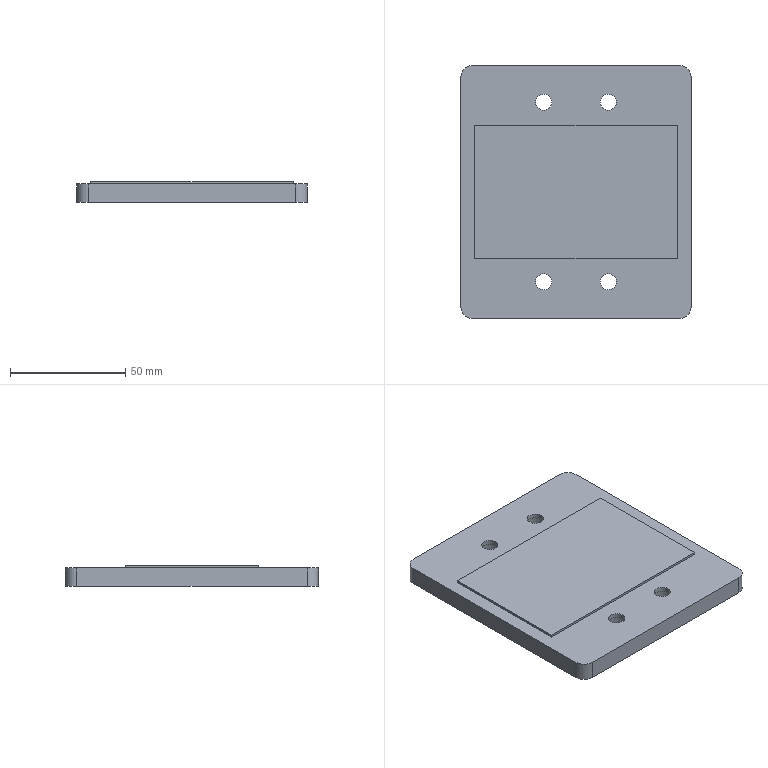Part | SolidWorks | features ICE 3, Extrusion 1 | 1 solid | 35 faces | box 100 x 110 x 9 mm | volume 89910 mm3 | cylinder 20 | plane 15 | commonest cylinder face diameters 7 x8 12 x8 10 x4
STEP:
#1=CARTESIAN_POINT('',(17.5,-39.,8.));
#2=VERTEX_POINT('',#1);
#3=CARTESIAN_POINT('',(10.5,-39.,8.));
#4=VERTEX_POINT('',#3);
#5=CARTESIAN_POINT('',(14.,-39.,8.));
#6=DIRECTION('',(0.,0.,-1.));
#7=DIRECTION('',(-1.,0.,0.));
#8=AXIS2_PLACEMENT_3D('',#5,#6,#7);
#9=CIRCLE('',#8,3.5);
#10=EDGE_CURVE('',#2,#4,#9,.T.);
#11=ORIENTED_EDGE('',*,*,#10,.F.);
#12=CARTESIAN_POINT('',(17.5,-39.,6.));
#13=VERTEX_POINT('',#12);
#14=CARTESIAN_POINT('',(17.5,-39.,12.));
#15=DIRECTION('',(0.,0.,-1.));
#16=VECTOR('',#15,1000.);
#17=LINE('',#14,#16);
#18=EDGE_CURVE('',#2,#13,#17,.T.);
#19=ORIENTED_EDGE('',*,*,#18,.T.);
#20=CARTESIAN_POINT('',(10.5,-39.,6.));
#21=VERTEX_POINT('',#20);
#22=CARTESIAN_POINT('',(14.,-39.,6.));
#23=DIRECTION('',(0.,0.,-1.));
#24=DIRECTION('',(1.,0.,0.));
#25=AXIS2_PLACEMENT_3D('',#22,#23,#24);
#26=CIRCLE('',#25,3.5);
#27=EDGE_CURVE('',#13,#21,#26,.T.);
#28=ORIENTED_EDGE('',*,*,#27,.T.);
#29=CARTESIAN_POINT('',(10.5,-39.,12.));
#30=DIRECTION('',(0.,0.,-1.));
#31=VECTOR('',#30,1000.);
#32=LINE('',#29,#31);
#33=EDGE_CURVE('',#4,#21,#32,.T.);
#34=ORIENTED_EDGE('',*,*,#33,.F.);
#35=EDGE_LOOP('',(#11,#19,#28,#34));
#36=FACE_OUTER_BOUND('',#35,.T.);
#37=CARTESIAN_POINT('',(14.,-39.,12.));
#38=DIRECTION('',(0.,0.,-1.));
#39=DIRECTION('',(-1.,0.,0.));
#40=AXIS2_PLACEMENT_3D('',#37,#38,#39);
#41=CYLINDRICAL_SURFACE('',#40,3.5);
#42=ADVANCED_FACE('',(#36),#41,.F.);
#43=CARTESIAN_POINT('',(-10.5,-39.,8.));
#44=VERTEX_POINT('',#43);
#45=CARTESIAN_POINT('',(-17.5,-39.,8.));
#46=VERTEX_POINT('',#45);
#47=CARTESIAN_POINT('',(-14.,-39.,8.));
#48=DIRECTION('',(0.,0.,-1.));
#49=DIRECTION('',(-1.,0.,0.));
#50=AXIS2_PLACEMENT_3D('',#47,#48,#49);
#51=CIRCLE('',#50,3.5);
#52=EDGE_CURVE('',#44,#46,#51,.T.);
#53=ORIENTED_EDGE('',*,*,#52,.F.);
#54=CARTESIAN_POINT('',(-10.5,-39.,6.));
#55=VERTEX_POINT('',#54);
#56=CARTESIAN_POINT('',(-10.5,-39.,12.));
#57=DIRECTION('',(0.,0.,-1.));
#58=VECTOR('',#57,1000.);
#59=LINE('',#56,#58);
#60=EDGE_CURVE('',#44,#55,#59,.T.);
#61=ORIENTED_EDGE('',*,*,#60,.T.);
#62=CARTESIAN_POINT('',(-17.5,-39.,6.));
#63=VERTEX_POINT('',#62);
#64=CARTESIAN_POINT('',(-14.,-39.,6.));
#65=DIRECTION('',(0.,0.,-1.));
#66=DIRECTION('',(1.,0.,0.));
#67=AXIS2_PLACEMENT_3D('',#64,#65,#66);
#68=CIRCLE('',#67,3.5);
#69=EDGE_CURVE('',#55,#63,#68,.T.);
#70=ORIENTED_EDGE('',*,*,#69,.T.);
#71=CARTESIAN_POINT('',(-17.5,-39.,12.));
#72=DIRECTION('',(0.,0.,-1.));
#73=VECTOR('',#72,1000.);
#74=LINE('',#71,#73);
#75=EDGE_CURVE('',#46,#63,#74,.T.);
#76=ORIENTED_EDGE('',*,*,#75,.F.);
#77=EDGE_LOOP('',(#53,#61,#70,#76));
#78=FACE_OUTER_BOUND('',#77,.T.);
#79=CARTESIAN_POINT('',(-14.,-39.,12.));
#80=DIRECTION('',(0.,0.,-1.));
#81=DIRECTION('',(-1.,0.,0.));
#82=AXIS2_PLACEMENT_3D('',#79,#80,#81);
#83=CYLINDRICAL_SURFACE('',#82,3.5);
#84=ADVANCED_FACE('',(#78),#83,.F.);
#85=CARTESIAN_POINT('',(-10.5,39.,8.));
#86=VERTEX_POINT('',#85);
#87=CARTESIAN_POINT('',(-17.5,39.,8.));
#88=VERTEX_POINT('',#87);
#89=CARTESIAN_POINT('',(-14.,39.,8.));
#90=DIRECTION('',(0.,0.,-1.));
#91=DIRECTION('',(-1.,0.,0.));
#92=AXIS2_PLACEMENT_3D('',#89,#90,#91);
#93=CIRCLE('',#92,3.5);
#94=EDGE_CURVE('',#86,#88,#93,.T.);
#95=ORIENTED_EDGE('',*,*,#94,.F.);
#96=CARTESIAN_POINT('',(-10.5,39.,6.));
#97=VERTEX_POINT('',#96);
#98=CARTESIAN_POINT('',(-10.5,39.,12.));
#99=DIRECTION('',(0.,0.,-1.));
#100=VECTOR('',#99,1000.);
#101=LINE('',#98,#100);
#102=EDGE_CURVE('',#86,#97,#101,.T.);
#103=ORIENTED_EDGE('',*,*,#102,.T.);
#104=CARTESIAN_POINT('',(-17.5,39.,6.));
#105=VERTEX_POINT('',#104);
#106=CARTESIAN_POINT('',(-14.,39.,6.));
#107=DIRECTION('',(0.,0.,-1.));
#108=DIRECTION('',(-1.,0.,0.));
#109=AXIS2_PLACEMENT_3D('',#106,#107,#108);
#110=CIRCLE('',#109,3.5);
#111=EDGE_CURVE('',#97,#105,#110,.T.);
#112=ORIENTED_EDGE('',*,*,#111,.T.);
#113=CARTESIAN_POINT('',(-17.5,39.,12.));
#114=DIRECTION('',(0.,0.,-1.));
#115=VECTOR('',#114,1000.);
#116=LINE('',#113,#115);
#117=EDGE_CURVE('',#88,#105,#116,.T.);
#118=ORIENTED_EDGE('',*,*,#117,.F.);
#119=EDGE_LOOP('',(#95,#103,#112,#118));
#120=FACE_OUTER_BOUND('',#119,.T.);
#121=CARTESIAN_POINT('',(-14.,39.,12.));
#122=DIRECTION('',(0.,0.,-1.));
#123=DIRECTION('',(-1.,0.,0.));
#124=AXIS2_PLACEMENT_3D('',#121,#122,#123);
#125=CYLINDRICAL_SURFACE('',#124,3.5);
#126=ADVANCED_FACE('',(#120),#125,.F.);
#127=CARTESIAN_POINT('',(17.5,39.,8.));
#128=VERTEX_POINT('',#127);
#129=CARTESIAN_POINT('',(10.5,39.,8.));
#130=VERTEX_POINT('',#129);
#131=CARTESIAN_POINT('',(14.,39.,8.));
#132=DIRECTION('',(0.,0.,-1.));
#133=DIRECTION('',(-1.,0.,0.));
#134=AXIS2_PLACEMENT_3D('',#131,#132,#133);
#135=CIRCLE('',#134,3.5);
#136=EDGE_CURVE('',#128,#130,#135,.T.);
#137=ORIENTED_EDGE('',*,*,#136,.F.);
#138=CARTESIAN_POINT('',(17.5,39.,6.));
#139=VERTEX_POINT('',#138);
#140=CARTESIAN_POINT('',(17.5,39.,12.));
#141=DIRECTION('',(0.,0.,-1.));
#142=VECTOR('',#141,1000.);
#143=LINE('',#140,#142);
#144=EDGE_CURVE('',#128,#139,#143,.T.);
#145=ORIENTED_EDGE('',*,*,#144,.T.);
#146=CARTESIAN_POINT('',(10.5,39.,6.));
#147=VERTEX_POINT('',#146);
#148=CARTESIAN_POINT('',(14.,39.,6.));
#149=DIRECTION('',(0.,0.,-1.));
#150=DIRECTION('',(-1.,0.,0.));
#151=AXIS2_PLACEMENT_3D('',#148,#149,#150);
#152=CIRCLE('',#151,3.5);
#153=EDGE_CURVE('',#139,#147,#152,.T.);
#154=ORIENTED_EDGE('',*,*,#153,.T.);
#155=CARTESIAN_POINT('',(10.5,39.,12.));
#156=DIRECTION('',(0.,0.,-1.));
#157=VECTOR('',#156,1000.);
#158=LINE('',#155,#157);
#159=EDGE_CURVE('',#130,#147,#158,.T.);
#160=ORIENTED_EDGE('',*,*,#159,.F.);
#161=EDGE_LOOP('',(#137,#145,#154,#160));
#162=FACE_OUTER_BOUND('',#161,.T.);
#163=CARTESIAN_POINT('',(14.,39.,12.));
#164=DIRECTION('',(0.,0.,-1.));
#165=DIRECTION('',(-1.,0.,0.));
#166=AXIS2_PLACEMENT_3D('',#163,#164,#165);
#167=CYLINDRICAL_SURFACE('',#166,3.5);
#168=ADVANCED_FACE('',(#162),#167,.F.);
#169=CARTESIAN_POINT('',(20.,39.,6.));
#170=VERTEX_POINT('',#169);
#171=CARTESIAN_POINT('',(8.,39.,6.));
#172=VERTEX_POINT('',#171);
#173=CARTESIAN_POINT('',(14.,39.,6.));
#174=DIRECTION('',(0.,0.,-1.));
#175=DIRECTION('',(1.,0.,0.));
#176=AXIS2_PLACEMENT_3D('',#173,#174,#175);
#177=CIRCLE('',#176,6.);
#178=EDGE_CURVE('',#170,#172,#177,.T.);
#179=ORIENTED_EDGE('',*,*,#178,.F.);
#180=CARTESIAN_POINT('',(20.,39.,0.));
#181=VERTEX_POINT('',#180);
#182=CARTESIAN_POINT('',(20.,39.,6.));
#183=DIRECTION('',(0.,0.,-1.));
#184=VECTOR('',#183,1000.);
#185=LINE('',#182,#184);
#186=EDGE_CURVE('',#170,#181,#185,.T.);
#187=ORIENTED_EDGE('',*,*,#186,.T.);
#188=CARTESIAN_POINT('',(8.,39.,0.));
#189=VERTEX_POINT('',#188);
#190=CARTESIAN_POINT('',(14.,39.,0.));
#191=DIRECTION('',(0.,0.,-1.));
#192=DIRECTION('',(1.,0.,0.));
#193=AXIS2_PLACEMENT_3D('',#190,#191,#192);
#194=CIRCLE('',#193,6.);
#195=EDGE_CURVE('',#181,#189,#194,.T.);
#196=ORIENTED_EDGE('',*,*,#195,.T.);
#197=CARTESIAN_POINT('',(8.,39.,6.));
#198=DIRECTION('',(0.,0.,-1.));
#199=VECTOR('',#198,1000.);
#200=LINE('',#197,#199);
#201=EDGE_CURVE('',#172,#189,#200,.T.);
#202=ORIENTED_EDGE('',*,*,#201,.F.);
#203=EDGE_LOOP('',(#179,#187,#196,#202));
#204=FACE_OUTER_BOUND('',#203,.T.);
#205=CARTESIAN_POINT('',(14.,39.,6.));
#206=DIRECTION('',(0.,0.,-1.));
#207=DIRECTION('',(-1.,0.,0.));
#208=AXIS2_PLACEMENT_3D('',#205,#206,#207);
#209=CYLINDRICAL_SURFACE('',#208,6.);
#210=ADVANCED_FACE('',(#204),#209,.F.);
#211=CARTESIAN_POINT('',(-8.,39.,6.));
#212=VERTEX_POINT('',#211);
#213=CARTESIAN_POINT('',(-20.,39.,6.));
#214=VERTEX_POINT('',#213);
#215=CARTESIAN_POINT('',(-14.,39.,6.));
#216=DIRECTION('',(0.,0.,-1.));
#217=DIRECTION('',(1.,0.,0.));
#218=AXIS2_PLACEMENT_3D('',#215,#216,#217);
#219=CIRCLE('',#218,6.);
#220=EDGE_CURVE('',#212,#214,#219,.T.);
#221=ORIENTED_EDGE('',*,*,#220,.F.);
#222=CARTESIAN_POINT('',(-8.,39.,0.));
#223=VERTEX_POINT('',#222);
#224=CARTESIAN_POINT('',(-8.,39.,6.));
#225=DIRECTION('',(0.,0.,-1.));
#226=VECTOR('',#225,1000.);
#227=LINE('',#224,#226);
#228=EDGE_CURVE('',#212,#223,#227,.T.);
#229=ORIENTED_EDGE('',*,*,#228,.T.);
#230=CARTESIAN_POINT('',(-20.,39.,0.));
#231=VERTEX_POINT('',#230);
#232=CARTESIAN_POINT('',(-14.,39.,0.));
#233=DIRECTION('',(0.,0.,-1.));
#234=DIRECTION('',(1.,0.,0.));
#235=AXIS2_PLACEMENT_3D('',#232,#233,#234);
#236=CIRCLE('',#235,6.);
#237=EDGE_CURVE('',#223,#231,#236,.T.);
#238=ORIENTED_EDGE('',*,*,#237,.T.);
#239=CARTESIAN_POINT('',(-20.,39.,6.));
#240=DIRECTION('',(0.,0.,-1.));
#241=VECTOR('',#240,1000.);
#242=LINE('',#239,#241);
#243=EDGE_CURVE('',#214,#231,#242,.T.);
#244=ORIENTED_EDGE('',*,*,#243,.F.);
#245=EDGE_LOOP('',(#221,#229,#238,#244));
#246=FACE_OUTER_BOUND('',#245,.T.);
#247=CARTESIAN_POINT('',(-14.,39.,6.));
#248=DIRECTION('',(0.,0.,-1.));
#249=DIRECTION('',(-1.,0.,0.));
#250=AXIS2_PLACEMENT_3D('',#247,#248,#249);
#251=CYLINDRICAL_SURFACE('',#250,6.);
#252=ADVANCED_FACE('',(#246),#251,.F.);
#253=CARTESIAN_POINT('',(-8.,-39.,6.));
#254=VERTEX_POINT('',#253);
#255=CARTESIAN_POINT('',(-20.,-39.,6.));
#256=VERTEX_POINT('',#255);
#257=CARTESIAN_POINT('',(-14.,-39.,6.));
#258=DIRECTION('',(0.,0.,-1.));
#259=DIRECTION('',(-1.,0.,0.));
#260=AXIS2_PLACEMENT_3D('',#257,#258,#259);
#261=CIRCLE('',#260,6.);
#262=EDGE_CURVE('',#254,#256,#261,.T.);
#263=ORIENTED_EDGE('',*,*,#262,.F.);
#264=CARTESIAN_POINT('',(-8.,-39.,0.));
#265=VERTEX_POINT('',#264);
#266=CARTESIAN_POINT('',(-8.,-39.,6.));
#267=DIRECTION('',(0.,0.,-1.));
#268=VECTOR('',#267,1000.);
#269=LINE('',#266,#268);
#270=EDGE_CURVE('',#254,#265,#269,.T.);
#271=ORIENTED_EDGE('',*,*,#270,.T.);
#272=CARTESIAN_POINT('',(-20.,-39.,0.));
#273=VERTEX_POINT('',#272);
#274=CARTESIAN_POINT('',(-14.,-39.,0.));
#275=DIRECTION('',(0.,0.,-1.));
#276=DIRECTION('',(-1.,0.,0.));
#277=AXIS2_PLACEMENT_3D('',#274,#275,#276);
#278=CIRCLE('',#277,6.);
#279=EDGE_CURVE('',#265,#273,#278,.T.);
#280=ORIENTED_EDGE('',*,*,#279,.T.);
#281=CARTESIAN_POINT('',(-20.,-39.,6.));
#282=DIRECTION('',(0.,0.,-1.));
#283=VECTOR('',#282,1000.);
#284=LINE('',#281,#283);
#285=EDGE_CURVE('',#256,#273,#284,.T.);
#286=ORIENTED_EDGE('',*,*,#285,.F.);
#287=EDGE_LOOP('',(#263,#271,#280,#286));
#288=FACE_OUTER_BOUND('',#287,.T.);
#289=CARTESIAN_POINT('',(-14.,-39.,6.));
#290=DIRECTION('',(0.,0.,-1.));
#291=DIRECTION('',(-1.,0.,0.));
#292=AXIS2_PLACEMENT_3D('',#289,#290,#291);
#293=CYLINDRICAL_SURFACE('',#292,6.);
#294=ADVANCED_FACE('',(#288),#293,.F.);
#295=CARTESIAN_POINT('',(20.,-39.,6.));
#296=VERTEX_POINT('',#295);
#297=CARTESIAN_POINT('',(8.,-39.,6.));
#298=VERTEX_POINT('',#297);
#299=CARTESIAN_POINT('',(14.,-39.,6.));
#300=DIRECTION('',(0.,0.,-1.));
#301=DIRECTION('',(-1.,0.,0.));
#302=AXIS2_PLACEMENT_3D('',#299,#300,#301);
#303=CIRCLE('',#302,6.);
#304=EDGE_CURVE('',#296,#298,#303,.T.);
#305=ORIENTED_EDGE('',*,*,#304,.F.);
#306=CARTESIAN_POINT('',(20.,-39.,0.));
#307=VERTEX_POINT('',#306);
#308=CARTESIAN_POINT('',(20.,-39.,6.));
#309=DIRECTION('',(0.,0.,-1.));
#310=VECTOR('',#309,1000.);
#311=LINE('',#308,#310);
#312=EDGE_CURVE('',#296,#307,#311,.T.);
#313=ORIENTED_EDGE('',*,*,#312,.T.);
#314=CARTESIAN_POINT('',(8.,-39.,0.));
#315=VERTEX_POINT('',#314);
#316=CARTESIAN_POINT('',(14.,-39.,0.));
#317=DIRECTION('',(0.,0.,-1.));
#318=DIRECTION('',(-1.,0.,0.));
#319=AXIS2_PLACEMENT_3D('',#316,#317,#318);
#320=CIRCLE('',#319,6.);
#321=EDGE_CURVE('',#307,#315,#320,.T.);
#322=ORIENTED_EDGE('',*,*,#321,.T.);
#323=CARTESIAN_POINT('',(8.,-39.,6.));
#324=DIRECTION('',(0.,0.,-1.));
#325=VECTOR('',#324,1000.);
#326=LINE('',#323,#325);
#327=EDGE_CURVE('',#298,#315,#326,.T.);
#328=ORIENTED_EDGE('',*,*,#327,.F.);
#329=EDGE_LOOP('',(#305,#313,#322,#328));
#330=FACE_OUTER_BOUND('',#329,.T.);
#331=CARTESIAN_POINT('',(14.,-39.,6.));
#332=DIRECTION('',(0.,0.,-1.));
#333=DIRECTION('',(-1.,0.,0.));
#334=AXIS2_PLACEMENT_3D('',#331,#332,#333);
#335=CYLINDRICAL_SURFACE('',#334,6.);
#336=ADVANCED_FACE('',(#330),#335,.F.);
#337=CARTESIAN_POINT('',(14.,-39.,8.));
#338=DIRECTION('',(0.,0.,-1.));
#339=DIRECTION('',(-1.,0.,0.));
#340=AXIS2_PLACEMENT_3D('',#337,#338,#339);
#341=CIRCLE('',#340,3.5);
#342=EDGE_CURVE('',#4,#2,#341,.T.);
#343=ORIENTED_EDGE('',*,*,#342,.T.);
#344=ORIENTED_EDGE('',*,*,#10,.T.);
#345=EDGE_LOOP('',(#343,#344));
#346=FACE_BOUND('',#345,.T.);
#347=CARTESIAN_POINT('',(-14.,-39.,8.));
#348=DIRECTION('',(0.,0.,-1.));
#349=DIRECTION('',(-1.,0.,0.));
#350=AXIS2_PLACEMENT_3D('',#347,#348,#349);
#351=CIRCLE('',#350,3.5);
#352=EDGE_CURVE('',#46,#44,#351,.T.);
#353=ORIENTED_EDGE('',*,*,#352,.T.);
#354=ORIENTED_EDGE('',*,*,#52,.T.);
#355=EDGE_LOOP('',(#353,#354));
#356=FACE_BOUND('',#355,.T.);
#357=CARTESIAN_POINT('',(-14.,39.,8.));
#358=DIRECTION('',(0.,0.,-1.));
#359=DIRECTION('',(-1.,0.,0.));
#360=AXIS2_PLACEMENT_3D('',#357,#358,#359);
#361=CIRCLE('',#360,3.5);
#362=EDGE_CURVE('',#88,#86,#361,.T.);
#363=ORIENTED_EDGE('',*,*,#362,.T.);
#364=ORIENTED_EDGE('',*,*,#94,.T.);
#365=EDGE_LOOP('',(#363,#364));
#366=FACE_BOUND('',#365,.T.);
#367=CARTESIAN_POINT('',(14.,39.,8.));
#368=DIRECTION('',(0.,0.,-1.));
#369=DIRECTION('',(-1.,0.,0.));
#370=AXIS2_PLACEMENT_3D('',#367,#368,#369);
#371=CIRCLE('',#370,3.5);
#372=EDGE_CURVE('',#130,#128,#371,.T.);
#373=ORIENTED_EDGE('',*,*,#372,.T.);
#374=ORIENTED_EDGE('',*,*,#136,.T.);
#375=EDGE_LOOP('',(#373,#374));
#376=FACE_BOUND('',#375,.T.);
#377=CARTESIAN_POINT('',(-50.,-50.,8.));
#378=VERTEX_POINT('',#377);
#379=CARTESIAN_POINT('',(-45.,-55.,8.));
#380=VERTEX_POINT('',#379);
#381=CARTESIAN_POINT('',(-45.,-50.,8.));
#382=DIRECTION('',(0.,0.,1.));
#383=DIRECTION('',(-1.,0.,0.));
#384=AXIS2_PLACEMENT_3D('',#381,#382,#383);
#385=CIRCLE('',#384,5.);
#386=EDGE_CURVE('',#378,#380,#385,.T.);
#387=ORIENTED_EDGE('',*,*,#386,.T.);
#388=CARTESIAN_POINT('',(45.,-55.,8.));
#389=VERTEX_POINT('',#388);
#390=CARTESIAN_POINT('',(-45.,-55.,8.));
#391=DIRECTION('',(1.,0.,0.));
#392=VECTOR('',#391,1000.);
#393=LINE('',#390,#392);
#394=EDGE_CURVE('',#380,#389,#393,.T.);
#395=ORIENTED_EDGE('',*,*,#394,.T.);
#396=CARTESIAN_POINT('',(50.,-50.,8.));
#397=VERTEX_POINT('',#396);
#398=CARTESIAN_POINT('',(45.,-50.,8.));
#399=DIRECTION('',(0.,0.,1.));
#400=DIRECTION('',(1.,0.,0.));
#401=AXIS2_PLACEMENT_3D('',#398,#399,#400);
#402=CIRCLE('',#401,5.);
#403=EDGE_CURVE('',#389,#397,#402,.T.);
#404=ORIENTED_EDGE('',*,*,#403,.T.);
#405=CARTESIAN_POINT('',(50.,50.,8.));
#406=VERTEX_POINT('',#405);
#407=CARTESIAN_POINT('',(50.,-50.,8.));
#408=DIRECTION('',(0.,1.,0.));
#409=VECTOR('',#408,1000.);
#410=LINE('',#407,#409);
#411=EDGE_CURVE('',#397,#406,#410,.T.);
#412=ORIENTED_EDGE('',*,*,#411,.T.);
#413=CARTESIAN_POINT('',(45.,55.,8.));
#414=VERTEX_POINT('',#413);
#415=CARTESIAN_POINT('',(45.,50.,8.));
#416=DIRECTION('',(0.,0.,1.));
#417=DIRECTION('',(-1.,0.,0.));
#418=AXIS2_PLACEMENT_3D('',#415,#416,#417);
#419=CIRCLE('',#418,5.);
#420=EDGE_CURVE('',#406,#414,#419,.T.);
#421=ORIENTED_EDGE('',*,*,#420,.T.);
#422=CARTESIAN_POINT('',(-45.,55.,8.));
#423=VERTEX_POINT('',#422);
#424=CARTESIAN_POINT('',(-45.,55.,8.));
#425=DIRECTION('',(-1.,0.,0.));
#426=VECTOR('',#425,1000.);
#427=LINE('',#424,#426);
#428=EDGE_CURVE('',#414,#423,#427,.T.);
#429=ORIENTED_EDGE('',*,*,#428,.T.);
#430=CARTESIAN_POINT('',(-50.,50.,8.));
#431=VERTEX_POINT('',#430);
#432=CARTESIAN_POINT('',(-45.,50.,8.));
#433=DIRECTION('',(0.,0.,1.));
#434=DIRECTION('',(-1.,0.,0.));
#435=AXIS2_PLACEMENT_3D('',#432,#433,#434);
#436=CIRCLE('',#435,5.);
#437=EDGE_CURVE('',#423,#431,#436,.T.);
#438=ORIENTED_EDGE('',*,*,#437,.T.);
#439=CARTESIAN_POINT('',(-50.,-50.,8.));
#440=DIRECTION('',(0.,-1.,0.));
#441=VECTOR('',#440,1000.);
#442=LINE('',#439,#441);
#443=EDGE_CURVE('',#431,#378,#442,.T.);
#444=ORIENTED_EDGE('',*,*,#443,.T.);
#445=EDGE_LOOP('',(#387,#395,#404,#412,#421,#429,#438,#444));
#446=FACE_OUTER_BOUND('',#445,.T.);
#447=CARTESIAN_POINT('',(44.,-29.,8.));
#448=VERTEX_POINT('',#447);
#449=CARTESIAN_POINT('',(44.,29.,8.));
#450=VERTEX_POINT('',#449);
#451=CARTESIAN_POINT('',(44.,-29.,8.));
#452=DIRECTION('',(0.,1.,0.));
#453=VECTOR('',#452,1000.);
#454=LINE('',#451,#453);
#455=EDGE_CURVE('',#448,#450,#454,.T.);
#456=ORIENTED_EDGE('',*,*,#455,.F.);
#457=CARTESIAN_POINT('',(-44.,-29.,8.));
#458=VERTEX_POINT('',#457);
#459=CARTESIAN_POINT('',(-44.,-29.,8.));
#460=DIRECTION('',(1.,0.,0.));
#461=VECTOR('',#460,1000.);
#462=LINE('',#459,#461);
#463=EDGE_CURVE('',#458,#448,#462,.T.);
#464=ORIENTED_EDGE('',*,*,#463,.F.);
#465=CARTESIAN_POINT('',(-44.,29.,8.));
#466=VERTEX_POINT('',#465);
#467=CARTESIAN_POINT('',(-44.,-29.,8.));
#468=DIRECTION('',(0.,-1.,0.));
#469=VECTOR('',#468,1000.);
#470=LINE('',#467,#469);
#471=EDGE_CURVE('',#466,#458,#470,.T.);
#472=ORIENTED_EDGE('',*,*,#471,.F.);
#473=CARTESIAN_POINT('',(-44.,29.,8.));
#474=DIRECTION('',(-1.,0.,0.));
#475=VECTOR('',#474,1000.);
#476=LINE('',#473,#475);
#477=EDGE_CURVE('',#450,#466,#476,.T.);
#478=ORIENTED_EDGE('',*,*,#477,.F.);
#479=EDGE_LOOP('',(#456,#464,#472,#478));
#480=FACE_BOUND('',#479,.T.);
#481=CARTESIAN_POINT('',(-45.,-50.,8.));
#482=DIRECTION('',(0.,0.,-1.));
#483=DIRECTION('',(-1.,0.,0.));
#484=AXIS2_PLACEMENT_3D('',#481,#482,#483);
#485=PLANE('',#484);
#486=ADVANCED_FACE('',(#346,#356,#366,#376,#446,#480),#485,.F.);
#487=CARTESIAN_POINT('',(-50.,-50.,0.));
#488=VERTEX_POINT('',#487);
#489=CARTESIAN_POINT('',(-45.,-55.,0.));
#490=VERTEX_POINT('',#489);
#491=CARTESIAN_POINT('',(-45.,-50.,0.));
#492=DIRECTION('',(0.,0.,1.));
#493=DIRECTION('',(-1.,0.,0.));
#494=AXIS2_PLACEMENT_3D('',#491,#492,#493);
#495=CIRCLE('',#494,5.);
#496=EDGE_CURVE('',#488,#490,#495,.T.);
#497=ORIENTED_EDGE('',*,*,#496,.T.);
#498=CARTESIAN_POINT('',(-45.,-55.,8.));
#499=DIRECTION('',(0.,0.,-1.));
#500=VECTOR('',#499,1000.);
#501=LINE('',#498,#500);
#502=EDGE_CURVE('',#380,#490,#501,.T.);
#503=ORIENTED_EDGE('',*,*,#502,.F.);
#504=ORIENTED_EDGE('',*,*,#386,.F.);
#505=CARTESIAN_POINT('',(-50.,-50.,8.));
#506=DIRECTION('',(0.,0.,-1.));
#507=VECTOR('',#506,1000.);
#508=LINE('',#505,#507);
#509=EDGE_CURVE('',#378,#488,#508,.T.);
#510=ORIENTED_EDGE('',*,*,#509,.T.);
#511=EDGE_LOOP('',(#497,#503,#504,#510));
#512=FACE_OUTER_BOUND('',#511,.T.);
#513=CARTESIAN_POINT('',(-45.,-50.,8.));
#514=DIRECTION('',(0.,0.,-1.));
#515=DIRECTION('',(-1.,0.,0.));
#516=AXIS2_PLACEMENT_3D('',#513,#514,#515);
#517=CYLINDRICAL_SURFACE('',#516,5.);
#518=ADVANCED_FACE('',(#512),#517,.T.);
#519=CARTESIAN_POINT('',(45.,-55.,0.));
#520=VERTEX_POINT('',#519);
#521=CARTESIAN_POINT('',(-45.,-55.,0.));
#522=DIRECTION('',(1.,0.,0.));
#523=VECTOR('',#522,1000.);
#524=LINE('',#521,#523);
#525=EDGE_CURVE('',#490,#520,#524,.T.);
#526=ORIENTED_EDGE('',*,*,#525,.T.);
#527=CARTESIAN_POINT('',(45.,-55.,8.));
#528=DIRECTION('',(0.,0.,-1.));
#529=VECTOR('',#528,1000.);
#530=LINE('',#527,#529);
#531=EDGE_CURVE('',#389,#520,#530,.T.);
#532=ORIENTED_EDGE('',*,*,#531,.F.);
#533=ORIENTED_EDGE('',*,*,#394,.F.);
#534=ORIENTED_EDGE('',*,*,#502,.T.);
#535=EDGE_LOOP('',(#526,#532,#533,#534));
#536=FACE_OUTER_BOUND('',#535,.T.);
#537=CARTESIAN_POINT('',(-45.,-55.,8.));
#538=DIRECTION('',(0.,1.,0.));
#539=DIRECTION('',(0.,0.,1.));
#540=AXIS2_PLACEMENT_3D('',#537,#538,#539);
#541=PLANE('',#540);
#542=ADVANCED_FACE('',(#536),#541,.F.);
#543=CARTESIAN_POINT('',(50.,-50.,0.));
#544=VERTEX_POINT('',#543);
#545=CARTESIAN_POINT('',(45.,-50.,0.));
#546=DIRECTION('',(0.,0.,1.));
#547=DIRECTION('',(1.,0.,0.));
#548=AXIS2_PLACEMENT_3D('',#545,#546,#547);
#549=CIRCLE('',#548,5.);
#550=EDGE_CURVE('',#520,#544,#549,.T.);
#551=ORIENTED_EDGE('',*,*,#550,.T.);
#552=CARTESIAN_POINT('',(50.,-50.,8.));
#553=DIRECTION('',(0.,0.,-1.));
#554=VECTOR('',#553,1000.);
#555=LINE('',#552,#554);
#556=EDGE_CURVE('',#397,#544,#555,.T.);
#557=ORIENTED_EDGE('',*,*,#556,.F.);
#558=ORIENTED_EDGE('',*,*,#403,.F.);
#559=ORIENTED_EDGE('',*,*,#531,.T.);
#560=EDGE_LOOP('',(#551,#557,#558,#559));
#561=FACE_OUTER_BOUND('',#560,.T.);
#562=CARTESIAN_POINT('',(45.,-50.,8.));
#563=DIRECTION('',(0.,0.,-1.));
#564=DIRECTION('',(-1.,0.,0.));
#565=AXIS2_PLACEMENT_3D('',#562,#563,#564);
#566=CYLINDRICAL_SURFACE('',#565,5.);
#567=ADVANCED_FACE('',(#561),#566,.T.);
#568=CARTESIAN_POINT('',(50.,50.,0.));
#569=VERTEX_POINT('',#568);
#570=CARTESIAN_POINT('',(50.,-50.,0.));
#571=DIRECTION('',(0.,1.,0.));
#572=VECTOR('',#571,1000.);
#573=LINE('',#570,#572);
#574=EDGE_CURVE('',#544,#569,#573,.T.);
#575=ORIENTED_EDGE('',*,*,#574,.T.);
#576=CARTESIAN_POINT('',(50.,50.,8.));
#577=DIRECTION('',(0.,0.,-1.));
#578=VECTOR('',#577,1000.);
#579=LINE('',#576,#578);
#580=EDGE_CURVE('',#406,#569,#579,.T.);
#581=ORIENTED_EDGE('',*,*,#580,.F.);
#582=ORIENTED_EDGE('',*,*,#411,.F.);
#583=ORIENTED_EDGE('',*,*,#556,.T.);
#584=EDGE_LOOP('',(#575,#581,#582,#583));
#585=FACE_OUTER_BOUND('',#584,.T.);
#586=CARTESIAN_POINT('',(50.,-50.,8.));
#587=DIRECTION('',(-1.,0.,0.));
#588=DIRECTION('',(0.,0.,1.));
#589=AXIS2_PLACEMENT_3D('',#586,#587,#588);
#590=PLANE('',#589);
#591=ADVANCED_FACE('',(#585),#590,.F.);
#592=CARTESIAN_POINT('',(45.,55.,0.));
#593=VERTEX_POINT('',#592);
#594=CARTESIAN_POINT('',(45.,50.,0.));
#595=DIRECTION('',(0.,0.,1.));
#596=DIRECTION('',(-1.,0.,0.));
#597=AXIS2_PLACEMENT_3D('',#594,#595,#596);
#598=CIRCLE('',#597,5.);
#599=EDGE_CURVE('',#569,#593,#598,.T.);
#600=ORIENTED_EDGE('',*,*,#599,.T.);
#601=CARTESIAN_POINT('',(45.,55.,8.));
#602=DIRECTION('',(0.,0.,-1.));
#603=VECTOR('',#602,1000.);
#604=LINE('',#601,#603);
#605=EDGE_CURVE('',#414,#593,#604,.T.);
#606=ORIENTED_EDGE('',*,*,#605,.F.);
#607=ORIENTED_EDGE('',*,*,#420,.F.);
#608=ORIENTED_EDGE('',*,*,#580,.T.);
#609=EDGE_LOOP('',(#600,#606,#607,#608));
#610=FACE_OUTER_BOUND('',#609,.T.);
#611=CARTESIAN_POINT('',(45.,50.,8.));
#612=DIRECTION('',(0.,0.,-1.));
#613=DIRECTION('',(-1.,0.,0.));
#614=AXIS2_PLACEMENT_3D('',#611,#612,#613);
#615=CYLINDRICAL_SURFACE('',#614,5.);
#616=ADVANCED_FACE('',(#610),#615,.T.);
#617=CARTESIAN_POINT('',(-45.,55.,0.));
#618=VERTEX_POINT('',#617);
#619=CARTESIAN_POINT('',(-45.,55.,0.));
#620=DIRECTION('',(-1.,0.,0.));
#621=VECTOR('',#620,1000.);
#622=LINE('',#619,#621);
#623=EDGE_CURVE('',#593,#618,#622,.T.);
#624=ORIENTED_EDGE('',*,*,#623,.T.);
#625=CARTESIAN_POINT('',(-45.,55.,8.));
#626=DIRECTION('',(0.,0.,-1.));
#627=VECTOR('',#626,1000.);
#628=LINE('',#625,#627);
#629=EDGE_CURVE('',#423,#618,#628,.T.);
#630=ORIENTED_EDGE('',*,*,#629,.F.);
#631=ORIENTED_EDGE('',*,*,#428,.F.);
#632=ORIENTED_EDGE('',*,*,#605,.T.);
#633=EDGE_LOOP('',(#624,#630,#631,#632));
#634=FACE_OUTER_BOUND('',#633,.T.);
#635=CARTESIAN_POINT('',(-45.,55.,8.));
#636=DIRECTION('',(0.,-1.,0.));
#637=DIRECTION('',(0.,0.,-1.));
#638=AXIS2_PLACEMENT_3D('',#635,#636,#637);
#639=PLANE('',#638);
#640=ADVANCED_FACE('',(#634),#639,.F.);
#641=CARTESIAN_POINT('',(-50.,50.,0.));
#642=VERTEX_POINT('',#641);
#643=CARTESIAN_POINT('',(-45.,50.,0.));
#644=DIRECTION('',(0.,0.,1.));
#645=DIRECTION('',(-1.,0.,0.));
#646=AXIS2_PLACEMENT_3D('',#643,#644,#645);
#647=CIRCLE('',#646,5.);
#648=EDGE_CURVE('',#618,#642,#647,.T.);
#649=ORIENTED_EDGE('',*,*,#648,.T.);
#650=CARTESIAN_POINT('',(-50.,50.,8.));
#651=DIRECTION('',(0.,0.,-1.));
#652=VECTOR('',#651,1000.);
#653=LINE('',#650,#652);
#654=EDGE_CURVE('',#431,#642,#653,.T.);
#655=ORIENTED_EDGE('',*,*,#654,.F.);
#656=ORIENTED_EDGE('',*,*,#437,.F.);
#657=ORIENTED_EDGE('',*,*,#629,.T.);
#658=EDGE_LOOP('',(#649,#655,#656,#657));
#659=FACE_OUTER_BOUND('',#658,.T.);
#660=CARTESIAN_POINT('',(-45.,50.,8.));
#661=DIRECTION('',(0.,0.,-1.));
#662=DIRECTION('',(-1.,0.,0.));
#663=AXIS2_PLACEMENT_3D('',#660,#661,#662);
#664=CYLINDRICAL_SURFACE('',#663,5.);
#665=ADVANCED_FACE('',(#659),#664,.T.);
#666=CARTESIAN_POINT('',(-50.,-50.,0.));
#667=DIRECTION('',(0.,-1.,0.));
#668=VECTOR('',#667,1000.);
#669=LINE('',#666,#668);
#670=EDGE_CURVE('',#642,#488,#669,.T.);
#671=ORIENTED_EDGE('',*,*,#670,.T.);
#672=ORIENTED_EDGE('',*,*,#509,.F.);
#673=ORIENTED_EDGE('',*,*,#443,.F.);
#674=ORIENTED_EDGE('',*,*,#654,.T.);
#675=EDGE_LOOP('',(#671,#672,#673,#674));
#676=FACE_OUTER_BOUND('',#675,.T.);
#677=CARTESIAN_POINT('',(-50.,-50.,8.));
#678=DIRECTION('',(1.,0.,0.));
#679=DIRECTION('',(0.,0.,-1.));
#680=AXIS2_PLACEMENT_3D('',#677,#678,#679);
#681=PLANE('',#680);
#682=ADVANCED_FACE('',(#676),#681,.F.);
#683=CARTESIAN_POINT('',(14.,39.,0.));
#684=DIRECTION('',(0.,0.,-1.));
#685=DIRECTION('',(1.,0.,0.));
#686=AXIS2_PLACEMENT_3D('',#683,#684,#685);
#687=CIRCLE('',#686,6.);
#688=EDGE_CURVE('',#189,#181,#687,.T.);
#689=ORIENTED_EDGE('',*,*,#688,.F.);
#690=ORIENTED_EDGE('',*,*,#195,.F.);
#691=EDGE_LOOP('',(#689,#690));
#692=FACE_BOUND('',#691,.T.);
#693=CARTESIAN_POINT('',(-14.,39.,0.));
#694=DIRECTION('',(0.,0.,-1.));
#695=DIRECTION('',(1.,0.,0.));
#696=AXIS2_PLACEMENT_3D('',#693,#694,#695);
#697=CIRCLE('',#696,6.);
#698=EDGE_CURVE('',#231,#223,#697,.T.);
#699=ORIENTED_EDGE('',*,*,#698,.F.);
#700=ORIENTED_EDGE('',*,*,#237,.F.);
#701=EDGE_LOOP('',(#699,#700));
#702=FACE_BOUND('',#701,.T.);
#703=CARTESIAN_POINT('',(-14.,-39.,0.));
#704=DIRECTION('',(0.,0.,-1.));
#705=DIRECTION('',(-1.,0.,0.));
#706=AXIS2_PLACEMENT_3D('',#703,#704,#705);
#707=CIRCLE('',#706,6.);
#708=EDGE_CURVE('',#273,#265,#707,.T.);
#709=ORIENTED_EDGE('',*,*,#708,.F.);
#710=ORIENTED_EDGE('',*,*,#279,.F.);
#711=EDGE_LOOP('',(#709,#710));
#712=FACE_BOUND('',#711,.T.);
#713=CARTESIAN_POINT('',(14.,-39.,0.));
#714=DIRECTION('',(0.,0.,-1.));
#715=DIRECTION('',(-1.,0.,0.));
#716=AXIS2_PLACEMENT_3D('',#713,#714,#715);
#717=CIRCLE('',#716,6.);
#718=EDGE_CURVE('',#315,#307,#717,.T.);
#719=ORIENTED_EDGE('',*,*,#718,.F.);
#720=ORIENTED_EDGE('',*,*,#321,.F.);
#721=EDGE_LOOP('',(#719,#720));
#722=FACE_BOUND('',#721,.T.);
#723=ORIENTED_EDGE('',*,*,#496,.F.);
#724=ORIENTED_EDGE('',*,*,#670,.F.);
#725=ORIENTED_EDGE('',*,*,#648,.F.);
#726=ORIENTED_EDGE('',*,*,#623,.F.);
#727=ORIENTED_EDGE('',*,*,#599,.F.);
#728=ORIENTED_EDGE('',*,*,#574,.F.);
#729=ORIENTED_EDGE('',*,*,#550,.F.);
#730=ORIENTED_EDGE('',*,*,#525,.F.);
#731=EDGE_LOOP('',(#723,#724,#725,#726,#727,#728,#729,#730));
#732=FACE_OUTER_BOUND('',#731,.T.);
#733=CARTESIAN_POINT('',(-45.,-50.,0.));
#734=DIRECTION('',(0.,0.,-1.));
#735=DIRECTION('',(-1.,0.,0.));
#736=AXIS2_PLACEMENT_3D('',#733,#734,#735);
#737=PLANE('',#736);
#738=ADVANCED_FACE('',(#692,#702,#712,#722,#732),#737,.T.);
#739=ORIENTED_EDGE('',*,*,#455,.T.);
#740=CARTESIAN_POINT('',(44.,29.,9.));
#741=VERTEX_POINT('',#740);
#742=CARTESIAN_POINT('',(44.,29.,9.));
#743=DIRECTION('',(0.,0.,-1.));
#744=VECTOR('',#743,1000.);
#745=LINE('',#742,#744);
#746=EDGE_CURVE('',#741,#450,#745,.T.);
#747=ORIENTED_EDGE('',*,*,#746,.F.);
#748=CARTESIAN_POINT('',(44.,-29.,9.));
#749=VERTEX_POINT('',#748);
#750=CARTESIAN_POINT('',(44.,-29.,9.));
#751=DIRECTION('',(0.,1.,0.));
#752=VECTOR('',#751,1000.);
#753=LINE('',#750,#752);
#754=EDGE_CURVE('',#749,#741,#753,.T.);
#755=ORIENTED_EDGE('',*,*,#754,.F.);
#756=CARTESIAN_POINT('',(44.,-29.,9.));
#757=DIRECTION('',(0.,0.,-1.));
#758=VECTOR('',#757,1000.);
#759=LINE('',#756,#758);
#760=EDGE_CURVE('',#749,#448,#759,.T.);
#761=ORIENTED_EDGE('',*,*,#760,.T.);
#762=EDGE_LOOP('',(#739,#747,#755,#761));
#763=FACE_OUTER_BOUND('',#762,.T.);
#764=CARTESIAN_POINT('',(44.,-29.,9.));
#765=DIRECTION('',(-1.,0.,0.));
#766=DIRECTION('',(0.,0.,1.));
#767=AXIS2_PLACEMENT_3D('',#764,#765,#766);
#768=PLANE('',#767);
#769=ADVANCED_FACE('',(#763),#768,.F.);
#770=ORIENTED_EDGE('',*,*,#477,.T.);
#771=CARTESIAN_POINT('',(-44.,29.,9.));
#772=VERTEX_POINT('',#771);
#773=CARTESIAN_POINT('',(-44.,29.,9.));
#774=DIRECTION('',(0.,0.,-1.));
#775=VECTOR('',#774,1000.);
#776=LINE('',#773,#775);
#777=EDGE_CURVE('',#772,#466,#776,.T.);
#778=ORIENTED_EDGE('',*,*,#777,.F.);
#779=CARTESIAN_POINT('',(-44.,29.,9.));
#780=DIRECTION('',(-1.,0.,0.));
#781=VECTOR('',#780,1000.);
#782=LINE('',#779,#781);
#783=EDGE_CURVE('',#741,#772,#782,.T.);
#784=ORIENTED_EDGE('',*,*,#783,.F.);
#785=ORIENTED_EDGE('',*,*,#746,.T.);
#786=EDGE_LOOP('',(#770,#778,#784,#785));
#787=FACE_OUTER_BOUND('',#786,.T.);
#788=CARTESIAN_POINT('',(-44.,29.,9.));
#789=DIRECTION('',(0.,-1.,0.));
#790=DIRECTION('',(0.,0.,-1.));
#791=AXIS2_PLACEMENT_3D('',#788,#789,#790);
#792=PLANE('',#791);
#793=ADVANCED_FACE('',(#787),#792,.F.);
#794=ORIENTED_EDGE('',*,*,#471,.T.);
#795=CARTESIAN_POINT('',(-44.,-29.,9.));
#796=VERTEX_POINT('',#795);
#797=CARTESIAN_POINT('',(-44.,-29.,9.));
#798=DIRECTION('',(0.,0.,-1.));
#799=VECTOR('',#798,1000.);
#800=LINE('',#797,#799);
#801=EDGE_CURVE('',#796,#458,#800,.T.);
#802=ORIENTED_EDGE('',*,*,#801,.F.);
#803=CARTESIAN_POINT('',(-44.,-29.,9.));
#804=DIRECTION('',(0.,-1.,0.));
#805=VECTOR('',#804,1000.);
#806=LINE('',#803,#805);
#807=EDGE_CURVE('',#772,#796,#806,.T.);
#808=ORIENTED_EDGE('',*,*,#807,.F.);
#809=ORIENTED_EDGE('',*,*,#777,.T.);
#810=EDGE_LOOP('',(#794,#802,#808,#809));
#811=FACE_OUTER_BOUND('',#810,.T.);
#812=CARTESIAN_POINT('',(-44.,-29.,9.));
#813=DIRECTION('',(1.,0.,0.));
#814=DIRECTION('',(0.,0.,-1.));
#815=AXIS2_PLACEMENT_3D('',#812,#813,#814);
#816=PLANE('',#815);
#817=ADVANCED_FACE('',(#811),#816,.F.);
#818=ORIENTED_EDGE('',*,*,#463,.T.);
#819=ORIENTED_EDGE('',*,*,#760,.F.);
#820=CARTESIAN_POINT('',(-44.,-29.,9.));
#821=DIRECTION('',(1.,0.,0.));
#822=VECTOR('',#821,1000.);
#823=LINE('',#820,#822);
#824=EDGE_CURVE('',#796,#749,#823,.T.);
#825=ORIENTED_EDGE('',*,*,#824,.F.);
#826=ORIENTED_EDGE('',*,*,#801,.T.);
#827=EDGE_LOOP('',(#818,#819,#825,#826));
#828=FACE_OUTER_BOUND('',#827,.T.);
#829=CARTESIAN_POINT('',(-44.,-29.,9.));
#830=DIRECTION('',(0.,1.,0.));
#831=DIRECTION('',(0.,0.,1.));
#832=AXIS2_PLACEMENT_3D('',#829,#830,#831);
#833=PLANE('',#832);
#834=ADVANCED_FACE('',(#828),#833,.F.);
#835=ORIENTED_EDGE('',*,*,#754,.T.);
#836=ORIENTED_EDGE('',*,*,#783,.T.);
#837=ORIENTED_EDGE('',*,*,#807,.T.);
#838=ORIENTED_EDGE('',*,*,#824,.T.);
#839=EDGE_LOOP('',(#835,#836,#837,#838));
#840=FACE_OUTER_BOUND('',#839,.T.);
#841=CARTESIAN_POINT('',(0.,0.,9.));
#842=DIRECTION('',(0.,0.,-1.));
#843=DIRECTION('',(-1.,0.,0.));
#844=AXIS2_PLACEMENT_3D('',#841,#842,#843);
#845=PLANE('',#844);
#846=ADVANCED_FACE('',(#840),#845,.F.);
#847=ORIENTED_EDGE('',*,*,#312,.F.);
#848=CARTESIAN_POINT('',(14.,-39.,6.));
#849=DIRECTION('',(0.,0.,-1.));
#850=DIRECTION('',(-1.,0.,0.));
#851=AXIS2_PLACEMENT_3D('',#848,#849,#850);
#852=CIRCLE('',#851,6.);
#853=EDGE_CURVE('',#298,#296,#852,.T.);
#854=ORIENTED_EDGE('',*,*,#853,.F.);
#855=ORIENTED_EDGE('',*,*,#327,.T.);
#856=ORIENTED_EDGE('',*,*,#718,.T.);
#857=EDGE_LOOP('',(#847,#854,#855,#856));
#858=FACE_OUTER_BOUND('',#857,.T.);
#859=CARTESIAN_POINT('',(14.,-39.,6.));
#860=DIRECTION('',(0.,0.,-1.));
#861=DIRECTION('',(-1.,0.,0.));
#862=AXIS2_PLACEMENT_3D('',#859,#860,#861);
#863=CYLINDRICAL_SURFACE('',#862,6.);
#864=ADVANCED_FACE('',(#858),#863,.F.);
#865=CARTESIAN_POINT('',(14.,-39.,6.));
#866=DIRECTION('',(0.,0.,-1.));
#867=DIRECTION('',(1.,0.,0.));
#868=AXIS2_PLACEMENT_3D('',#865,#866,#867);
#869=CIRCLE('',#868,3.5);
#870=EDGE_CURVE('',#21,#13,#869,.T.);
#871=ORIENTED_EDGE('',*,*,#870,.F.);
#872=ORIENTED_EDGE('',*,*,#27,.F.);
#873=EDGE_LOOP('',(#871,#872));
#874=FACE_BOUND('',#873,.T.);
#875=ORIENTED_EDGE('',*,*,#853,.T.);
#876=ORIENTED_EDGE('',*,*,#304,.T.);
#877=EDGE_LOOP('',(#875,#876));
#878=FACE_OUTER_BOUND('',#877,.T.);
#879=CARTESIAN_POINT('',(14.,-39.,6.));
#880=DIRECTION('',(0.,0.,-1.));
#881=DIRECTION('',(-1.,0.,0.));
#882=AXIS2_PLACEMENT_3D('',#879,#880,#881);
#883=PLANE('',#882);
#884=ADVANCED_FACE('',(#874,#878),#883,.T.);
#885=ORIENTED_EDGE('',*,*,#270,.F.);
#886=CARTESIAN_POINT('',(-14.,-39.,6.));
#887=DIRECTION('',(0.,0.,-1.));
#888=DIRECTION('',(-1.,0.,0.));
#889=AXIS2_PLACEMENT_3D('',#886,#887,#888);
#890=CIRCLE('',#889,6.);
#891=EDGE_CURVE('',#256,#254,#890,.T.);
#892=ORIENTED_EDGE('',*,*,#891,.F.);
#893=ORIENTED_EDGE('',*,*,#285,.T.);
#894=ORIENTED_EDGE('',*,*,#708,.T.);
#895=EDGE_LOOP('',(#885,#892,#893,#894));
#896=FACE_OUTER_BOUND('',#895,.T.);
#897=CARTESIAN_POINT('',(-14.,-39.,6.));
#898=DIRECTION('',(0.,0.,-1.));
#899=DIRECTION('',(-1.,0.,0.));
#900=AXIS2_PLACEMENT_3D('',#897,#898,#899);
#901=CYLINDRICAL_SURFACE('',#900,6.);
#902=ADVANCED_FACE('',(#896),#901,.F.);
#903=CARTESIAN_POINT('',(-14.,-39.,6.));
#904=DIRECTION('',(0.,0.,-1.));
#905=DIRECTION('',(1.,0.,0.));
#906=AXIS2_PLACEMENT_3D('',#903,#904,#905);
#907=CIRCLE('',#906,3.5);
#908=EDGE_CURVE('',#63,#55,#907,.T.);
#909=ORIENTED_EDGE('',*,*,#908,.F.);
#910=ORIENTED_EDGE('',*,*,#69,.F.);
#911=EDGE_LOOP('',(#909,#910));
#912=FACE_BOUND('',#911,.T.);
#913=ORIENTED_EDGE('',*,*,#891,.T.);
#914=ORIENTED_EDGE('',*,*,#262,.T.);
#915=EDGE_LOOP('',(#913,#914));
#916=FACE_OUTER_BOUND('',#915,.T.);
#917=CARTESIAN_POINT('',(-14.,-39.,6.));
#918=DIRECTION('',(0.,0.,-1.));
#919=DIRECTION('',(-1.,0.,0.));
#920=AXIS2_PLACEMENT_3D('',#917,#918,#919);
#921=PLANE('',#920);
#922=ADVANCED_FACE('',(#912,#916),#921,.T.);
#923=ORIENTED_EDGE('',*,*,#228,.F.);
#924=CARTESIAN_POINT('',(-14.,39.,6.));
#925=DIRECTION('',(0.,0.,-1.));
#926=DIRECTION('',(1.,0.,0.));
#927=AXIS2_PLACEMENT_3D('',#924,#925,#926);
#928=CIRCLE('',#927,6.);
#929=EDGE_CURVE('',#214,#212,#928,.T.);
#930=ORIENTED_EDGE('',*,*,#929,.F.);
#931=ORIENTED_EDGE('',*,*,#243,.T.);
#932=ORIENTED_EDGE('',*,*,#698,.T.);
#933=EDGE_LOOP('',(#923,#930,#931,#932));
#934=FACE_OUTER_BOUND('',#933,.T.);
#935=CARTESIAN_POINT('',(-14.,39.,6.));
#936=DIRECTION('',(0.,0.,-1.));
#937=DIRECTION('',(-1.,0.,0.));
#938=AXIS2_PLACEMENT_3D('',#935,#936,#937);
#939=CYLINDRICAL_SURFACE('',#938,6.);
#940=ADVANCED_FACE('',(#934),#939,.F.);
#941=CARTESIAN_POINT('',(-14.,39.,6.));
#942=DIRECTION('',(0.,0.,-1.));
#943=DIRECTION('',(-1.,0.,0.));
#944=AXIS2_PLACEMENT_3D('',#941,#942,#943);
#945=CIRCLE('',#944,3.5);
#946=EDGE_CURVE('',#105,#97,#945,.T.);
#947=ORIENTED_EDGE('',*,*,#946,.F.);
#948=ORIENTED_EDGE('',*,*,#111,.F.);
#949=EDGE_LOOP('',(#947,#948));
#950=FACE_BOUND('',#949,.T.);
#951=ORIENTED_EDGE('',*,*,#929,.T.);
#952=ORIENTED_EDGE('',*,*,#220,.T.);
#953=EDGE_LOOP('',(#951,#952));
#954=FACE_OUTER_BOUND('',#953,.T.);
#955=CARTESIAN_POINT('',(-14.,39.,6.));
#956=DIRECTION('',(0.,0.,1.));
#957=DIRECTION('',(1.,0.,0.));
#958=AXIS2_PLACEMENT_3D('',#955,#956,#957);
#959=PLANE('',#958);
#960=ADVANCED_FACE('',(#950,#954),#959,.F.);
#961=ORIENTED_EDGE('',*,*,#186,.F.);
#962=CARTESIAN_POINT('',(14.,39.,6.));
#963=DIRECTION('',(0.,0.,-1.));
#964=DIRECTION('',(1.,0.,0.));
#965=AXIS2_PLACEMENT_3D('',#962,#963,#964);
#966=CIRCLE('',#965,6.);
#967=EDGE_CURVE('',#172,#170,#966,.T.);
#968=ORIENTED_EDGE('',*,*,#967,.F.);
#969=ORIENTED_EDGE('',*,*,#201,.T.);
#970=ORIENTED_EDGE('',*,*,#688,.T.);
#971=EDGE_LOOP('',(#961,#968,#969,#970));
#972=FACE_OUTER_BOUND('',#971,.T.);
#973=CARTESIAN_POINT('',(14.,39.,6.));
#974=DIRECTION('',(0.,0.,-1.));
#975=DIRECTION('',(-1.,0.,0.));
#976=AXIS2_PLACEMENT_3D('',#973,#974,#975);
#977=CYLINDRICAL_SURFACE('',#976,6.);
#978=ADVANCED_FACE('',(#972),#977,.F.);
#979=CARTESIAN_POINT('',(14.,39.,6.));
#980=DIRECTION('',(0.,0.,-1.));
#981=DIRECTION('',(-1.,0.,0.));
#982=AXIS2_PLACEMENT_3D('',#979,#980,#981);
#983=CIRCLE('',#982,3.5);
#984=EDGE_CURVE('',#147,#139,#983,.T.);
#985=ORIENTED_EDGE('',*,*,#984,.F.);
#986=ORIENTED_EDGE('',*,*,#153,.F.);
#987=EDGE_LOOP('',(#985,#986));
#988=FACE_BOUND('',#987,.T.);
#989=ORIENTED_EDGE('',*,*,#967,.T.);
#990=ORIENTED_EDGE('',*,*,#178,.T.);
#991=EDGE_LOOP('',(#989,#990));
#992=FACE_OUTER_BOUND('',#991,.T.);
#993=CARTESIAN_POINT('',(14.,39.,6.));
#994=DIRECTION('',(0.,0.,1.));
#995=DIRECTION('',(1.,0.,0.));
#996=AXIS2_PLACEMENT_3D('',#993,#994,#995);
#997=PLANE('',#996);
#998=ADVANCED_FACE('',(#988,#992),#997,.F.);
#999=ORIENTED_EDGE('',*,*,#144,.F.);
#1000=ORIENTED_EDGE('',*,*,#372,.F.);
#1001=ORIENTED_EDGE('',*,*,#159,.T.);
#1002=ORIENTED_EDGE('',*,*,#984,.T.);
#1003=EDGE_LOOP('',(#999,#1000,#1001,#1002));
#1004=FACE_OUTER_BOUND('',#1003,.T.);
#1005=CARTESIAN_POINT('',(14.,39.,12.));
#1006=DIRECTION('',(0.,0.,-1.));
#1007=DIRECTION('',(-1.,0.,0.));
#1008=AXIS2_PLACEMENT_3D('',#1005,#1006,#1007);
#1009=CYLINDRICAL_SURFACE('',#1008,3.5);
#1010=ADVANCED_FACE('',(#1004),#1009,.F.);
#1011=ORIENTED_EDGE('',*,*,#102,.F.);
#1012=ORIENTED_EDGE('',*,*,#362,.F.);
#1013=ORIENTED_EDGE('',*,*,#117,.T.);
#1014=ORIENTED_EDGE('',*,*,#946,.T.);
#1015=EDGE_LOOP('',(#1011,#1012,#1013,#1014));
#1016=FACE_OUTER_BOUND('',#1015,.T.);
#1017=CARTESIAN_POINT('',(-14.,39.,12.));
#1018=DIRECTION('',(0.,0.,-1.));
#1019=DIRECTION('',(-1.,0.,0.));
#1020=AXIS2_PLACEMENT_3D('',#1017,#1018,#1019);
#1021=CYLINDRICAL_SURFACE('',#1020,3.5);
#1022=ADVANCED_FACE('',(#1016),#1021,.F.);
#1023=ORIENTED_EDGE('',*,*,#60,.F.);
#1024=ORIENTED_EDGE('',*,*,#352,.F.);
#1025=ORIENTED_EDGE('',*,*,#75,.T.);
#1026=ORIENTED_EDGE('',*,*,#908,.T.);
#1027=EDGE_LOOP('',(#1023,#1024,#1025,#1026));
#1028=FACE_OUTER_BOUND('',#1027,.T.);
#1029=CARTESIAN_POINT('',(-14.,-39.,12.));
#1030=DIRECTION('',(0.,0.,-1.));
#1031=DIRECTION('',(-1.,0.,0.));
#1032=AXIS2_PLACEMENT_3D('',#1029,#1030,#1031);
#1033=CYLINDRICAL_SURFACE('',#1032,3.5);
#1034=ADVANCED_FACE('',(#1028),#1033,.F.);
#1035=ORIENTED_EDGE('',*,*,#18,.F.);
#1036=ORIENTED_EDGE('',*,*,#342,.F.);
#1037=ORIENTED_EDGE('',*,*,#33,.T.);
#1038=ORIENTED_EDGE('',*,*,#870,.T.);
#1039=EDGE_LOOP('',(#1035,#1036,#1037,#1038));
#1040=FACE_OUTER_BOUND('',#1039,.T.);
#1041=CARTESIAN_POINT('',(14.,-39.,12.));
#1042=DIRECTION('',(0.,0.,-1.));
#1043=DIRECTION('',(-1.,0.,0.));
#1044=AXIS2_PLACEMENT_3D('',#1041,#1042,#1043);
#1045=CYLINDRICAL_SURFACE('',#1044,3.5);
#1046=ADVANCED_FACE('',(#1040),#1045,.F.);
#1047=CLOSED_SHELL('',(#42,#84,#126,#168,#210,#252,#294,#336,#486,#518,#542,#567,#591,#616,#640,#665,#682,#738,#769,#793,#817,#834,#846,#864,#884,#902,#922,#940,#960,#978,#998,#1010,#1022,#1034,#1046));
#1048=MANIFOLD_SOLID_BREP('',#1047);
#1049=CARTESIAN_POINT('',(0.,0.,0.));
#1050=DIRECTION('',(0.,0.,1.));
#1051=DIRECTION('',(1.,0.,0.));
#1052=AXIS2_PLACEMENT_3D('',#1049,#1050,#1051);
#1053=(LENGTH_UNIT()NAMED_UNIT(*)SI_UNIT(.MILLI.,.METRE.));
#1054=UNCERTAINTY_MEASURE_WITH_UNIT(LENGTH_MEASURE(0.00001),#1053,'','');
#1055=(NAMED_UNIT(*)PLANE_ANGLE_UNIT()SI_UNIT($,.RADIAN.));
#1056=(NAMED_UNIT(*)SI_UNIT($,.STERADIAN.)SOLID_ANGLE_UNIT());
#1057=(GEOMETRIC_REPRESENTATION_CONTEXT(3)GLOBAL_UNCERTAINTY_ASSIGNED_CONTEXT((#1054))GLOBAL_UNIT_ASSIGNED_CONTEXT((#1053,#1055,#1056))REPRESENTATION_CONTEXT('',''));
#1058=ADVANCED_BREP_SHAPE_REPRESENTATION('',(#1048,#1052),#1057);